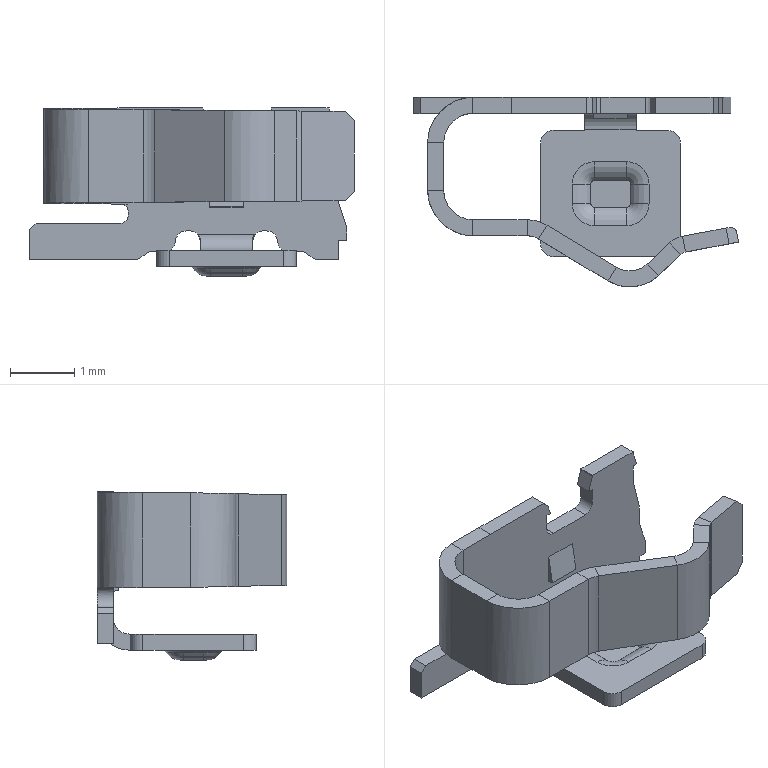Part | NX | 1 solid | 141 faces | box 5.066 x 2.959 x 2.622 mm | volume 5.787 mm3 | plane 89 | cylinder 38 | torus 12 | spline 2 | commonest cylinder face diameters 0.3 x6 0.2 x5 0.5 x5 0.7 x5 0.35 x4 0.4 x4